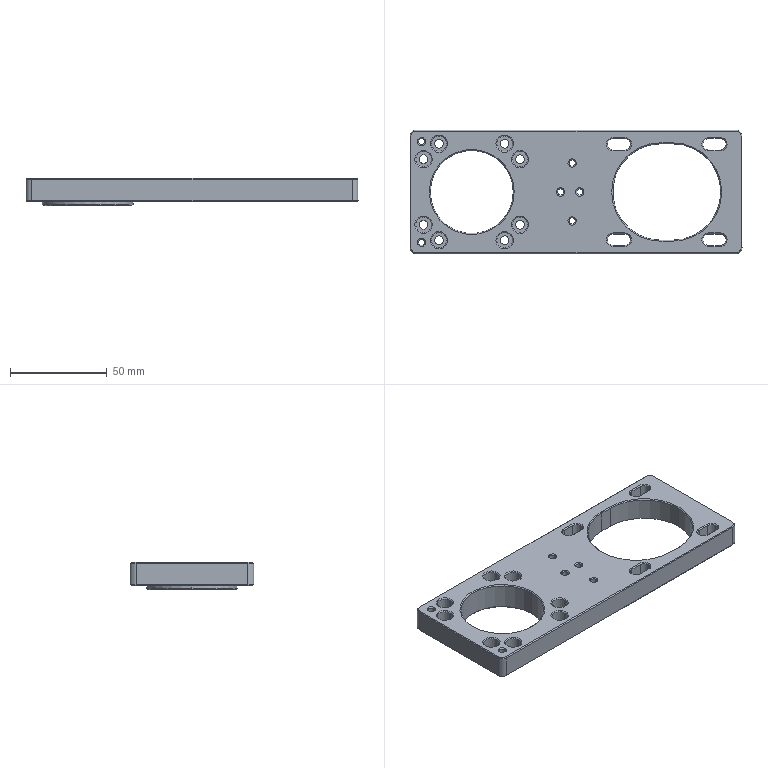Part | SolidWorks | features BaseBody 1 | 1 solid | 165 faces | box 172 x 64 x 14 mm | volume 80863 mm3 | cylinder 67 | cone 55 | plane 43 | commonest cylinder face diameters 4.5 x16 6 x16 8 x16 3.3 x12 50 x3 43 x2